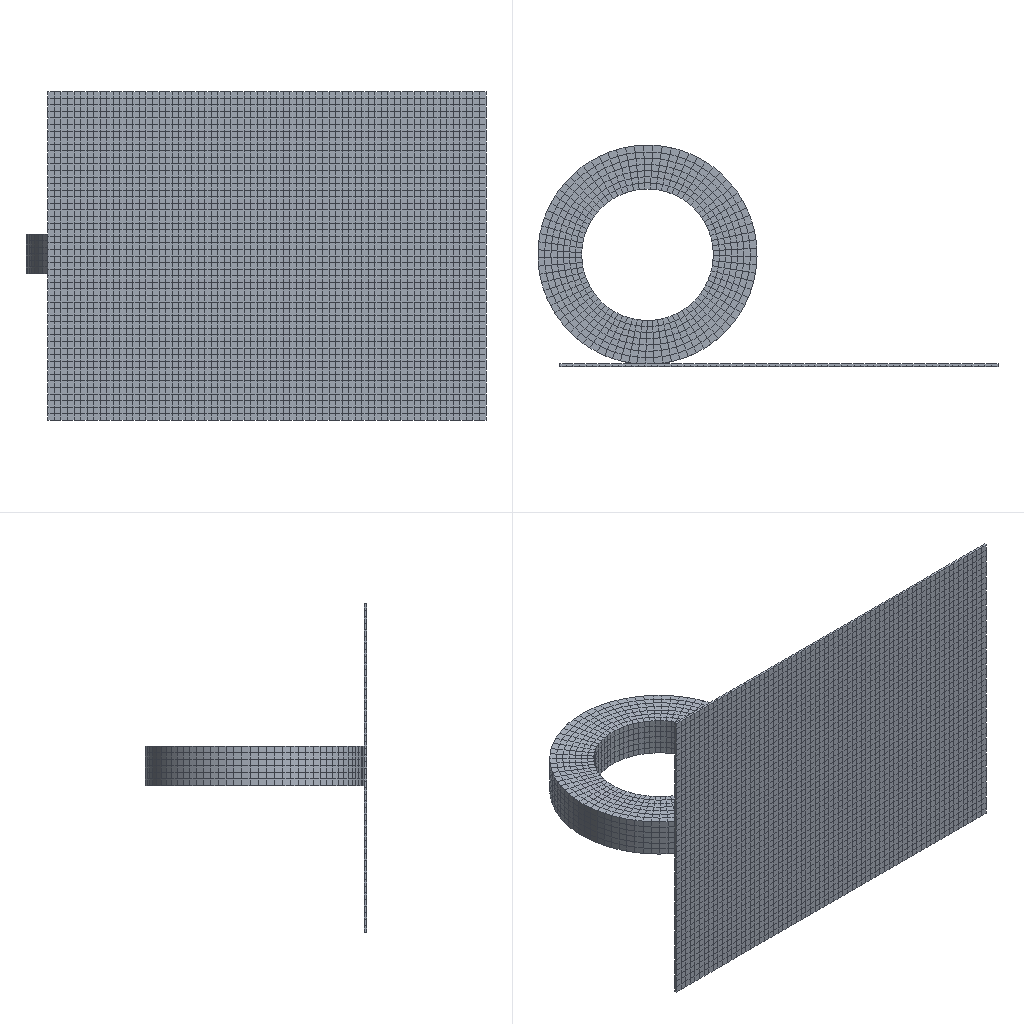Simulation study | abaqus
Set-up summary:
category,name,step,type,value,unit,region
solver,abaqus
solver,version,,,Abaqus/Standard 2020
units,not stated in the deck,,not stated
analysis,deck,,coupled temperature-displacement,coupled temperature-displacement
load_step,Step-1,Step-1,coupled temperature-displacement
load_step,Step-2,Step-2,coupled temperature-displacement
load_step,requested,,,2
mesh,nodes,,,11416
mesh,elements,,,6710
element_type,C3D8R,,solid,3350
element_type,C3D8RT,,solid,3360
load,load commands in deck,,count,3
bc,support commands in deck,,count,23
material,MATERIAL-1,,in results
check,setup vs results,,match,"per instance, exact: element labels, types and connectivity; labels of the nodes the elements use; coordinates of those nodes at SINGLE_PRECISION in 2 of 2 instance(s)"
Abaqus input file, long lists of numbers shortened:
*Heading
** Job name: Job-1 Model name: Model-1
** Generated by: Abaqus/CAE 2020
*Preprint, echo=NO, model=NO, history=NO, contact=NO
**
** PARTS
**
*Part, name=road
*Node
      1,           0.,        -150.,           1.
      2,           0.,        -147.,           1.
** (6934 more lines like these left out)
*Element, type=C3D8R
   1,  103,  104,  155,  154,    1,    2,   53,   52
   2,  104,  105,  156,  155,    2,    3,   54,   53
** (3348 more lines like these left out)
*Nset, nset=Set-1, generate
    1,  6936,     1
*Elset, elset=Set-1, generate
    1,  3350,     1
** Section: Section-1
*Solid Section, elset=Set-1, material=Material-1
,
*End Part
**
*Part, name=type
*Node
      1, -0.9732,  -49.991,           0.
      2,           0.,         -30.,           0.
** (4478 more lines like these left out)
*Element, type=C3D8RT
   1,  641,  651,  831,  680,    1,   11,  191,   40
   2,  651,  652,  832,  831,   11,   12,  192,  191
** (3358 more lines like these left out)
*Nset, nset=Set-1, generate
    1,  4480,     1
*Elset, elset=Set-1, generate
    1,  3360,     1
** Section: Section-1
*Solid Section, elset=Set-1, material=Material-1
,
*End Part
**
**
** ASSEMBLY
**
*Assembly, name=Assembly
**
*Instance, name=road-1, part=road
        -40.,         -50.,          83.
        -40.,         -50.,          83., -39.,         -50.,          83., 90.
*End Instance
**
*Instance, name=type-1, part=type
*End Instance
**
*Node
      1,           0.,           0.,           9.
*Node
      2,         160.,         -50.,           8.
*Nset, nset=Set-4
 1,
*Nset, nset=Set-5
 2,
*Nset, nset=Set-6
 1,
*Nset, nset=Set-7, instance=road-1, generate
    1,  6936,     1
*Nset, nset=Set-7, instance=type-1, generate
    1,  4480,     1
*Elset, elset=Set-7, instance=road-1, generate
    1,  3350,     1
*Elset, elset=Set-7, instance=type-1, generate
    1,  3360,     1
*Nset, nset=Set-8
 1,
*Nset, nset=b_Set-1, instance=road-1, generate
    1,  6936,     1
*Elset, elset=b_Set-1, instance=road-1, generate
    1,  3350,     1
*Nset, nset=m_Set-3
 1,
*Nset, nset=_PickedSet10, internal
 2,
*Elset, elset=_s_Surf-1_S4, internal, instance=type-1
    7,   14,   21,   28,   35,   42,   49,   56,   63,   70,   77,   84,   91,   98,  105,  112
  119,  126,  133,  140,  147,  154,  161,  168,  175,  182,  189,  196,  203,  567,  574,  581
** (9 more lines like these left out)
*Elset, elset=_s_Surf-1_S6, internal, instance=type-1
  204,  211,  218,  225,  232,  239,  246,  253,  260,  267,  274,  281,  288,  295,  302,  309
  316,  323,  330,  337,  344,  351,  358,  365,  372,  379,  386,  393,  400,  407,  414,  421
** (18 more lines like these left out)
*Surface, type=ELEMENT, name=s_Surf-1
_s_Surf-1_S4, S4
_s_Surf-1_S6, S6
** Constraint: Constraint-1
*Rigid Body, ref node=_PickedSet10, elset=b_Set-1
** Constraint: Constraint-2
*Coupling, constraint name=Constraint-2, ref node=m_Set-3, surface=s_Surf-1
*Kinematic
*Elset, elset=__Int-1_gcs0_7_S6, internal, instance=type-1
    1,    8,   15,   22,   29,   36,   43,   50,   57,   64,   71,   78,   85,   92,   99,  106
  113,  120,  127,  134,  141,  148,  155,  162,  169,  176,  183,  190,  197,  561,  568,  575
** (9 more lines like these left out)
*Elset, elset=__Int-1_gcs0_7_S4, internal, instance=type-1
  210,  217,  224,  231,  238,  245,  252,  259,  266,  273,  280,  287,  294,  301,  308,  315
  322,  329,  336,  343,  350,  357,  364,  371,  378,  385,  392,  399,  406,  413,  420,  427
** (18 more lines like these left out)
*Surface, type=ELEMENT, name=_Int-1_gcs0_7, internal
__Int-1_gcs0_7_S6, S6
__Int-1_gcs0_7_S4, S4
*Elset, elset=__Int-1_gcs0_8_S4, internal, instance=type-1
    7,   14,   21,   28,   35,   42,   49,   56,   63,   70,   77,   84,   91,   98,  105,  112
  119,  126,  133,  140,  147,  154,  161,  168,  175,  182,  189,  196,  203,  567,  574,  581
** (9 more lines like these left out)
*Elset, elset=__Int-1_gcs0_8_S6, internal, instance=type-1
  204,  211,  218,  225,  232,  239,  246,  253,  260,  267,  274,  281,  288,  295,  302,  309
  316,  323,  330,  337,  344,  351,  358,  365,  372,  379,  386,  393,  400,  407,  414,  421
** (18 more lines like these left out)
*Surface, type=ELEMENT, name=_Int-1_gcs0_8, internal
__Int-1_gcs0_8_S4, S4
__Int-1_gcs0_8_S6, S6
*End Assembly
*Amplitude, name=Amp-1
             0.,              0.,              1.,              1.
**
** MATERIALS
**
*Material, name=Material-1
*Conductivity
 0.2,
*Density
 1.13e-09,
*Elastic
1000., 0.4
*Expansion
 1.4e-05,
*Specific Heat
 1.57e+08,
**
** INTERACTION PROPERTIES
**
*Surface Interaction, name=IntProp-1
1.,
*Friction, slip tolerance=0.005
1.,
*Surface Behavior, pressure-overclosure=HARD
*Gap Conductance
 0.01,    0.
   0., 0.001
**
** PREDEFINED FIELDS
**
** Name: Predefined Field-1   Type: Temperature
*Initial Conditions, type=TEMPERATURE
Set-7, 20.
**
** INTERACTIONS
**
** Interaction: Int-1
*Contact
*Contact Inclusions, ALL EXTERIOR
*Contact Property Assignment
 ,  , IntProp-1
*Surface Property Assignment, property=GEOMETRIC CORRECTION
_Int-1_gcs0_7, Circumferential, 0., 0., 0.,  0., 0., 1.
_Int-1_gcs0_8, Circumferential, 0., 0., 0.,  0., 0., 1.
** ----------------------------------------------------------------
**
** STEP: Step-1
**
*Step, name=Step-1, nlgeom=YES, inc=1000
*Coupled Temperature-displacement, creep=none, deltmx=1e+12, stabilize=0.0002, allsdtol=0.05, continue=NO
0.01, 1., 1e-05, 1.
**
** BOUNDARY CONDITIONS
**
** Name: [REDACTED] : Displacement/rotation angle
*Boundary, amplitude=Amp-1
Set-5, 1, 1
Set-5, 2, 2, 2.
Set-5, 3, 3
Set-5, 4, 4
Set-5, 5, 5
Set-5, 6, 6
** Name: [REDACTED] : Displacement/rotation angle
*Boundary
Set-4, 1, 1
Set-4, 2, 2
Set-4, 3, 3
Set-4, 4, 4
Set-4, 5, 5
Set-4, 6, 6
**
** OUTPUT REQUESTS
**
*Restart, write, frequency=0
**
** FIELD OUTPUT: F-Output-1
**
*Output, field
*Node Output
CF, NT, RF, RFL, U, UR, UT, V
*Element Output, directions=YES
E, HFL, LE, MISES, MISESMAX, MISESONLY, PE, PEEQ, PEEQMAX, PEMAG, S, TEMP, YIELDPOT
*Contact Output
CDISP, CSTRESS
*Radiation Output
FTEMP,
**
** HISTORY OUTPUT: H-Output-1
**
*Output, history, variable=PRESELECT
*End Step
** ----------------------------------------------------------------
**
** STEP: Step-2
**
*Step, name=Step-2, nlgeom=YES, inc=10000
*Coupled Temperature-displacement, creep=none, deltmx=1e+10, stabilize=0.0002, allsdtol=0.05, continue=NO
0.01, 10., 1e-05, 1.
**
** BOUNDARY CONDITIONS
**
** Name: [REDACTED] : Displacement/rotation angle
*Boundary, op=NEW
Set-5, 1, 1
Set-5, 2, 2, 2.
Set-5, 3, 3
Set-5, 4, 4
Set-5, 5, 5
Set-5, 6, 6
** Name: [REDACTED] : Displacement/rotation angle
*Boundary, op=NEW
Set-4, 2, 2
Set-4, 3, 3
Set-4, 4, 4
Set-4, 5, 5
** Name: [REDACTED]
*Boundary, op=NEW, type=VELOCITY
Set-8, 6, 6, -0.3
**
** OUTPUT REQUESTS
**
*Restart, write, frequency=0
**
** FIELD OUTPUT: F-Output-1
**
*Output, field
*Node Output
CF, NT, RF, RFL, U, UR, UT, V
*Element Output, directions=YES
E, HFL, LE, MISES, MISESMAX, MISESONLY, PE, PEEQ, PEEQMAX, PEMAG, S, TEMP, YIELDPOT
*Contact Output
CDISP, CSTRESS
*Radiation Output
FTEMP,
**
** HISTORY OUTPUT: H-Output-1
**
*Output, history, variable=PRESELECT
*End Step
Results summary:
result,step,,completed,increments=14 time=1.0/1.0
result,step,,partial,increments=57 time=4.159/10.0
result,analysis,,,"coupled temperature-displacement, steady state"
result,last_loadstep,,,2
result,primary field,,,"U, NT11"
result,reaction total,,FX,0.5323,model units
result,reaction total,,FY,0.4414,model units
result,reaction total,,FZ,-0.0,model units